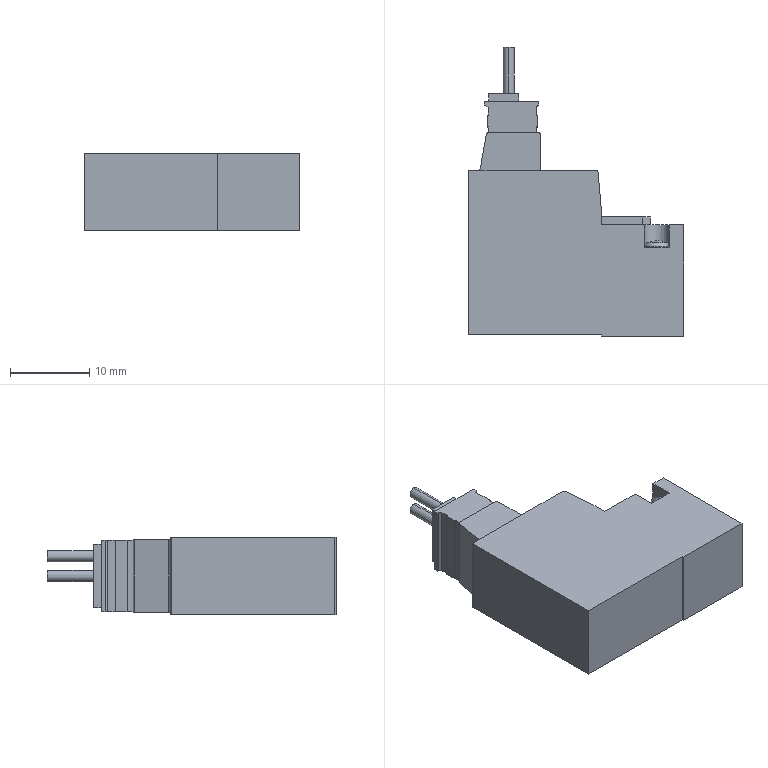Part | SolidWorks | features BaseBody 1 | 1 solid | 87 faces | box 27.2 x 36.5 x 9.8 mm | volume 5427 mm3 | plane 58 | cylinder 17 | cone 4 | torus 4 | sphere 4 | commonest cylinder face diameters 1.4 x4 3.2 x4 0.4 x3 0.6 x2 1.2 x2 3.4 x2